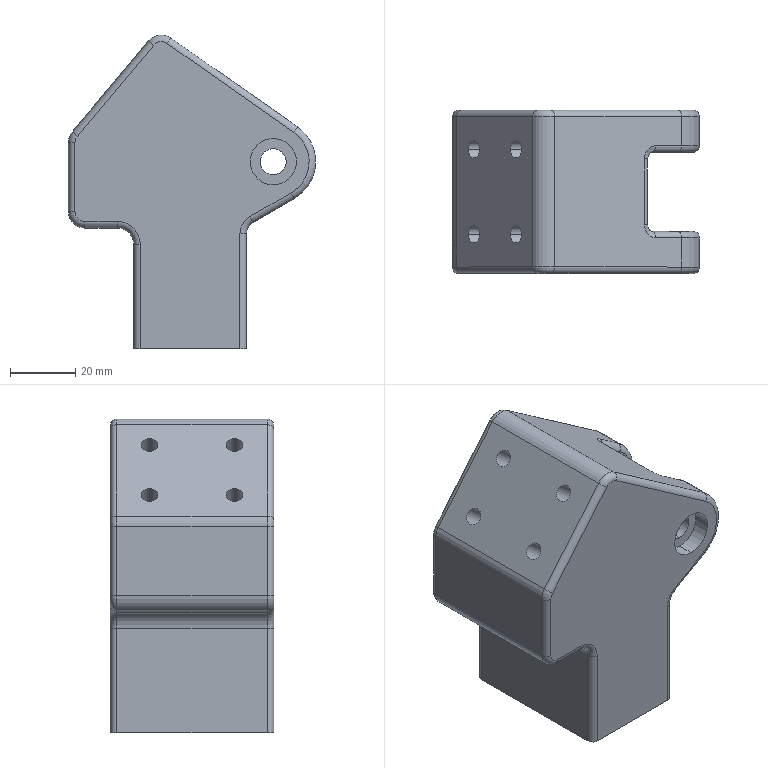Part | SolidWorks | features BaseBody 1 | 1 solid | 114 faces | box 75.712 x 50 x 96.074 mm | volume 193934 mm3 | cylinder 58 | plane 18 | cone 16 | torus 16 | spline 4 | sphere 2 | commonest cylinder face diameters 4 x26 5.2 x8 6.8 x8 7.95 x4 10 x4 14.2 x4